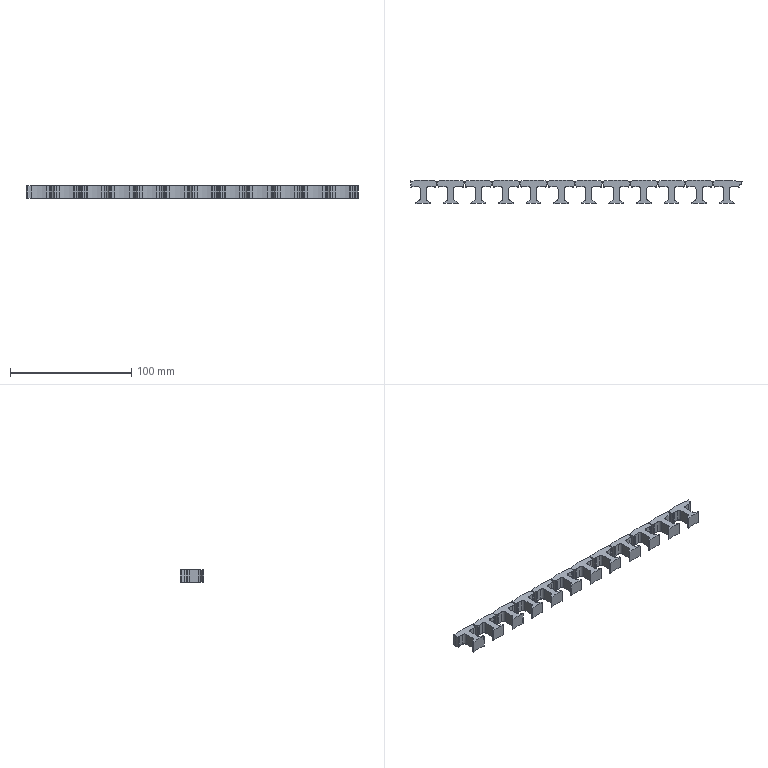Part | SolidWorks | features BaseBody 1 | 1 solid | 364 faces | box 273.994 x 19.727 x 10 mm | volume 23128 mm3 | cylinder 192 | plane 172 | commonest cylinder face diameters 4 x48 2 x36 1 x33 0.3 x24 79 x24 50 x12